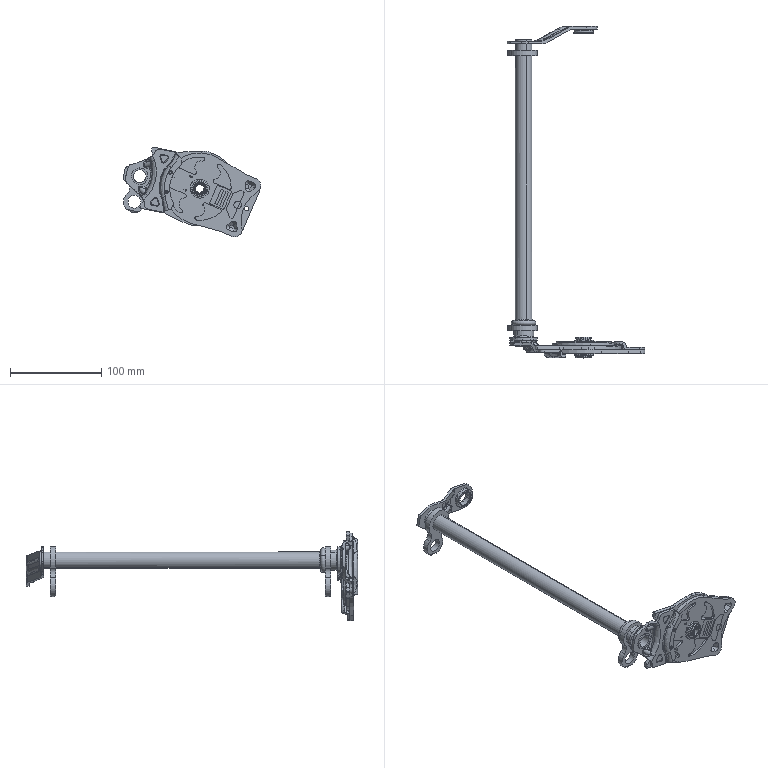Part | NX | features BREP 21 | 23 solids | 2428 faces | box 150.567 x 363 x 98.155 mm | volume 153864 mm3 | cylinder 916 | plane 657 | spline 436 | torus 219 | cone 168 | sphere 32 | commonest cylinder face diameters 0.3 x169 0.6 x144 1 x58 4 x40 2 x38 3 x32